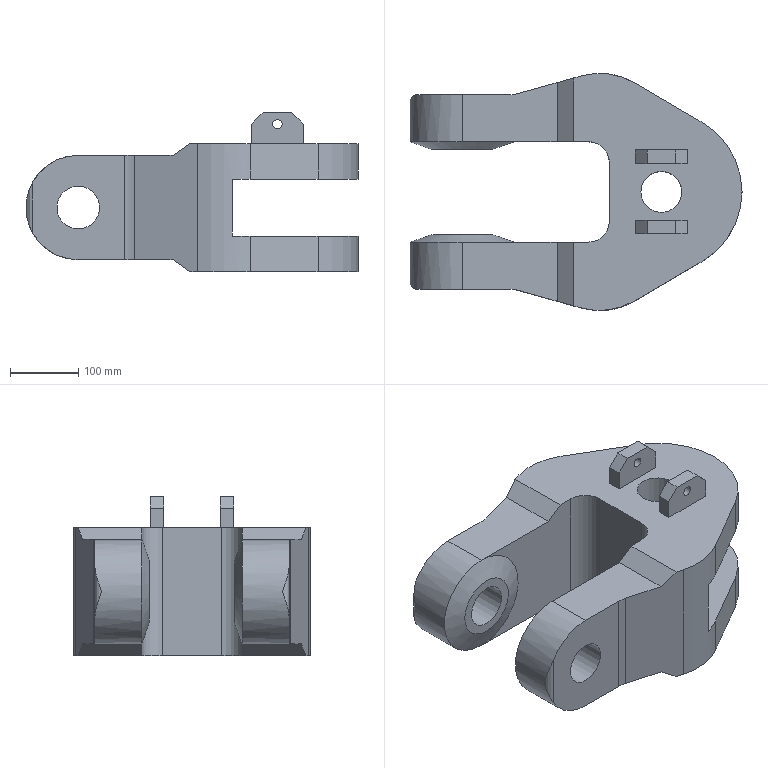Part | NX | features 推移杆连接头 2 | 1 solid | 60 faces | box 486.5 x 347.5 x 233.365 mm | volume 11889729 mm3 | plane 40 | cylinder 18 | cone 2 | commonest cylinder face diameters 60 x4 13.9 x2 20 x2 62.55 x2 100 x2 153 x2